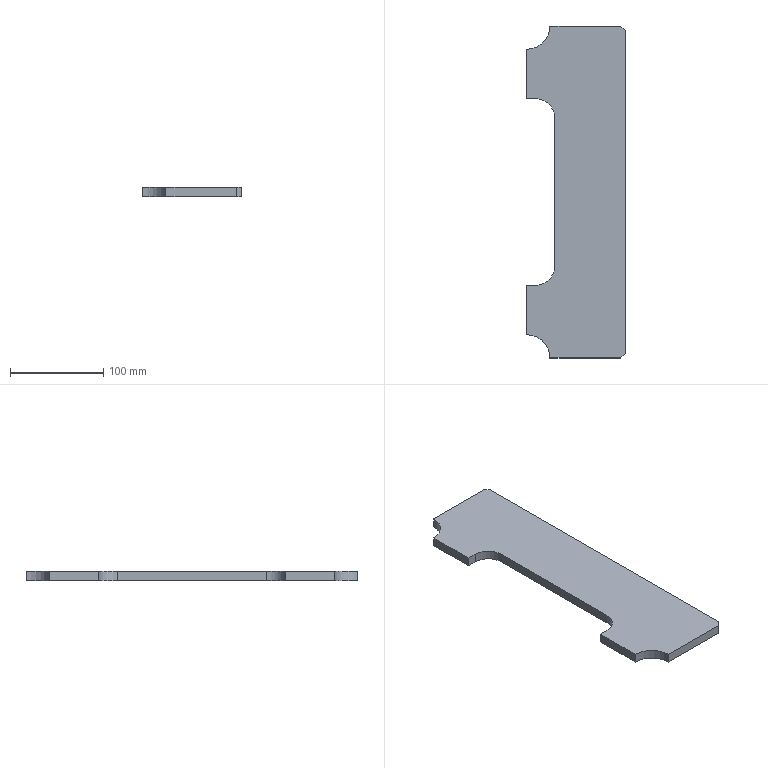Part | STEP file | VD-SYL0380DJ1006_1_1-9_VD-SYL03 | 1 solid | 16 faces | box 106 x 356 x 10 mm | volume 309009 mm3 | plane 12 | cylinder 4 | commonest cylinder face diameters 40 x2 50 x2
STEP:
#1=CARTESIAN_POINT('',(-53.,-153.,10.));
#2=VERTEX_POINT('',#1);
#3=CARTESIAN_POINT('',(-53.,-153.,0.));
#4=VERTEX_POINT('',#3);
#5=CARTESIAN_POINT('',(-53.,-153.,10.));
#6=DIRECTION('',(0.,0.,-1.));
#7=VECTOR('',#6,1000.);
#8=LINE('',#5,#7);
#9=EDGE_CURVE('',#2,#4,#8,.T.);
#10=ORIENTED_EDGE('',*,*,#9,.T.);
#11=CARTESIAN_POINT('',(-28.,-178.,0.));
#12=VERTEX_POINT('',#11);
#13=CARTESIAN_POINT('',(-53.,-178.,0.));
#14=DIRECTION('',(0.,0.,1.));
#15=DIRECTION('',(1.,0.,0.));
#16=AXIS2_PLACEMENT_3D('',#13,#14,#15);
#17=CIRCLE('',#16,25.);
#18=EDGE_CURVE('',#12,#4,#17,.T.);
#19=ORIENTED_EDGE('',*,*,#18,.F.);
#20=CARTESIAN_POINT('',(-28.,-178.,10.));
#21=VERTEX_POINT('',#20);
#22=CARTESIAN_POINT('',(-28.,-178.,0.));
#23=DIRECTION('',(0.,0.,1.));
#24=VECTOR('',#23,1000.);
#25=LINE('',#22,#24);
#26=EDGE_CURVE('',#12,#21,#25,.T.);
#27=ORIENTED_EDGE('',*,*,#26,.T.);
#28=CARTESIAN_POINT('',(-53.,-178.,10.));
#29=DIRECTION('',(0.,0.,-1.));
#30=DIRECTION('',(0.,1.,0.));
#31=AXIS2_PLACEMENT_3D('',#28,#29,#30);
#32=CIRCLE('',#31,25.);
#33=EDGE_CURVE('',#2,#21,#32,.T.);
#34=ORIENTED_EDGE('',*,*,#33,.F.);
#35=EDGE_LOOP('',(#10,#19,#27,#34));
#36=FACE_OUTER_BOUND('',#35,.T.);
#37=CARTESIAN_POINT('',(-53.,-178.,5.));
#38=DIRECTION('',(0.,0.,-1.));
#39=DIRECTION('',(-1.,0.,0.));
#40=AXIS2_PLACEMENT_3D('',#37,#38,#39);
#41=CYLINDRICAL_SURFACE('',#40,25.);
#42=ADVANCED_FACE('',(#36),#41,.F.);
#43=CARTESIAN_POINT('',(-43.,-100.,0.));
#44=VERTEX_POINT('',#43);
#45=CARTESIAN_POINT('',(-23.,-80.,0.));
#46=VERTEX_POINT('',#45);
#47=CARTESIAN_POINT('',(-43.,-80.,0.));
#48=DIRECTION('',(0.,0.,1.));
#49=DIRECTION('',(0.,-1.,0.));
#50=AXIS2_PLACEMENT_3D('',#47,#48,#49);
#51=CIRCLE('',#50,20.);
#52=EDGE_CURVE('',#44,#46,#51,.T.);
#53=ORIENTED_EDGE('',*,*,#52,.F.);
#54=CARTESIAN_POINT('',(-43.,-100.,10.));
#55=VERTEX_POINT('',#54);
#56=CARTESIAN_POINT('',(-43.,-100.,0.));
#57=DIRECTION('',(0.,0.,1.));
#58=VECTOR('',#57,1000.);
#59=LINE('',#56,#58);
#60=EDGE_CURVE('',#44,#55,#59,.T.);
#61=ORIENTED_EDGE('',*,*,#60,.T.);
#62=CARTESIAN_POINT('',(-23.,-80.,10.));
#63=VERTEX_POINT('',#62);
#64=CARTESIAN_POINT('',(-43.,-80.,10.));
#65=DIRECTION('',(0.,0.,-1.));
#66=DIRECTION('',(1.,0.,0.));
#67=AXIS2_PLACEMENT_3D('',#64,#65,#66);
#68=CIRCLE('',#67,20.);
#69=EDGE_CURVE('',#63,#55,#68,.T.);
#70=ORIENTED_EDGE('',*,*,#69,.F.);
#71=CARTESIAN_POINT('',(-23.,-80.,10.));
#72=DIRECTION('',(0.,0.,-1.));
#73=VECTOR('',#72,1000.);
#74=LINE('',#71,#73);
#75=EDGE_CURVE('',#63,#46,#74,.T.);
#76=ORIENTED_EDGE('',*,*,#75,.T.);
#77=EDGE_LOOP('',(#53,#61,#70,#76));
#78=FACE_OUTER_BOUND('',#77,.T.);
#79=CARTESIAN_POINT('',(-43.,-80.,-25.06));
#80=DIRECTION('',(0.,0.,1.));
#81=DIRECTION('',(1.,0.,0.));
#82=AXIS2_PLACEMENT_3D('',#79,#80,#81);
#83=CYLINDRICAL_SURFACE('',#82,20.);
#84=ADVANCED_FACE('',(#78),#83,.F.);
#85=CARTESIAN_POINT('',(-23.,80.,0.));
#86=VERTEX_POINT('',#85);
#87=CARTESIAN_POINT('',(-23.,80.,0.));
#88=DIRECTION('',(0.,-1.,0.));
#89=VECTOR('',#88,1000.);
#90=LINE('',#87,#89);
#91=EDGE_CURVE('',#86,#46,#90,.T.);
#92=ORIENTED_EDGE('',*,*,#91,.T.);
#93=ORIENTED_EDGE('',*,*,#75,.F.);
#94=CARTESIAN_POINT('',(-23.,80.,10.));
#95=VERTEX_POINT('',#94);
#96=CARTESIAN_POINT('',(-23.,-80.,10.));
#97=DIRECTION('',(0.,1.,0.));
#98=VECTOR('',#97,1000.);
#99=LINE('',#96,#98);
#100=EDGE_CURVE('',#63,#95,#99,.T.);
#101=ORIENTED_EDGE('',*,*,#100,.T.);
#102=CARTESIAN_POINT('',(-23.,80.,0.));
#103=DIRECTION('',(0.,0.,1.));
#104=VECTOR('',#103,1000.);
#105=LINE('',#102,#104);
#106=EDGE_CURVE('',#86,#95,#105,.T.);
#107=ORIENTED_EDGE('',*,*,#106,.F.);
#108=EDGE_LOOP('',(#92,#93,#101,#107));
#109=FACE_OUTER_BOUND('',#108,.T.);
#110=CARTESIAN_POINT('',(-23.,0.,5.));
#111=DIRECTION('',(1.,0.,0.));
#112=DIRECTION('',(0.,1.,0.));
#113=AXIS2_PLACEMENT_3D('',#110,#111,#112);
#114=PLANE('',#113);
#115=ADVANCED_FACE('',(#109),#114,.F.);
#116=CARTESIAN_POINT('',(-43.,100.,0.));
#117=VERTEX_POINT('',#116);
#118=CARTESIAN_POINT('',(-43.,80.,0.));
#119=DIRECTION('',(0.,0.,1.));
#120=DIRECTION('',(1.,0.,0.));
#121=AXIS2_PLACEMENT_3D('',#118,#119,#120);
#122=CIRCLE('',#121,20.);
#123=EDGE_CURVE('',#86,#117,#122,.T.);
#124=ORIENTED_EDGE('',*,*,#123,.F.);
#125=ORIENTED_EDGE('',*,*,#106,.T.);
#126=CARTESIAN_POINT('',(-43.,100.,10.));
#127=VERTEX_POINT('',#126);
#128=CARTESIAN_POINT('',(-43.,80.,10.));
#129=DIRECTION('',(0.,0.,-1.));
#130=DIRECTION('',(0.,1.,0.));
#131=AXIS2_PLACEMENT_3D('',#128,#129,#130);
#132=CIRCLE('',#131,20.);
#133=EDGE_CURVE('',#127,#95,#132,.T.);
#134=ORIENTED_EDGE('',*,*,#133,.F.);
#135=CARTESIAN_POINT('',(-43.,100.,10.));
#136=DIRECTION('',(0.,0.,-1.));
#137=VECTOR('',#136,1000.);
#138=LINE('',#135,#137);
#139=EDGE_CURVE('',#127,#117,#138,.T.);
#140=ORIENTED_EDGE('',*,*,#139,.T.);
#141=EDGE_LOOP('',(#124,#125,#134,#140));
#142=FACE_OUTER_BOUND('',#141,.T.);
#143=CARTESIAN_POINT('',(-43.,80.,-25.06));
#144=DIRECTION('',(0.,0.,1.));
#145=DIRECTION('',(1.,0.,0.));
#146=AXIS2_PLACEMENT_3D('',#143,#144,#145);
#147=CYLINDRICAL_SURFACE('',#146,20.);
#148=ADVANCED_FACE('',(#142),#147,.F.);
#149=CARTESIAN_POINT('',(-53.,100.,0.));
#150=VERTEX_POINT('',#149);
#151=CARTESIAN_POINT('',(-53.,100.,0.));
#152=DIRECTION('',(1.,0.,0.));
#153=VECTOR('',#152,1000.);
#154=LINE('',#151,#153);
#155=EDGE_CURVE('',#150,#117,#154,.T.);
#156=ORIENTED_EDGE('',*,*,#155,.T.);
#157=ORIENTED_EDGE('',*,*,#139,.F.);
#158=CARTESIAN_POINT('',(-53.,100.,10.));
#159=VERTEX_POINT('',#158);
#160=CARTESIAN_POINT('',(-43.,100.,10.));
#161=DIRECTION('',(-1.,0.,0.));
#162=VECTOR('',#161,1000.);
#163=LINE('',#160,#162);
#164=EDGE_CURVE('',#127,#159,#163,.T.);
#165=ORIENTED_EDGE('',*,*,#164,.T.);
#166=CARTESIAN_POINT('',(-53.,100.,10.));
#167=DIRECTION('',(0.,0.,-1.));
#168=VECTOR('',#167,1000.);
#169=LINE('',#166,#168);
#170=EDGE_CURVE('',#159,#150,#169,.T.);
#171=ORIENTED_EDGE('',*,*,#170,.T.);
#172=EDGE_LOOP('',(#156,#157,#165,#171));
#173=FACE_OUTER_BOUND('',#172,.T.);
#174=CARTESIAN_POINT('',(-38.,100.,5.));
#175=DIRECTION('',(0.,1.,0.));
#176=DIRECTION('',(1.,0.,0.));
#177=AXIS2_PLACEMENT_3D('',#174,#175,#176);
#178=PLANE('',#177);
#179=ADVANCED_FACE('',(#173),#178,.F.);
#180=CARTESIAN_POINT('',(-53.,153.,10.));
#181=VERTEX_POINT('',#180);
#182=CARTESIAN_POINT('',(-53.,100.,10.));
#183=DIRECTION('',(0.,1.,0.));
#184=VECTOR('',#183,1000.);
#185=LINE('',#182,#184);
#186=EDGE_CURVE('',#159,#181,#185,.T.);
#187=ORIENTED_EDGE('',*,*,#186,.T.);
#188=CARTESIAN_POINT('',(-53.,153.,0.));
#189=VERTEX_POINT('',#188);
#190=CARTESIAN_POINT('',(-53.,153.,0.));
#191=DIRECTION('',(0.,0.,1.));
#192=VECTOR('',#191,1000.);
#193=LINE('',#190,#192);
#194=EDGE_CURVE('',#189,#181,#193,.T.);
#195=ORIENTED_EDGE('',*,*,#194,.F.);
#196=CARTESIAN_POINT('',(-53.,153.,0.));
#197=DIRECTION('',(0.,-1.,0.));
#198=VECTOR('',#197,1000.);
#199=LINE('',#196,#198);
#200=EDGE_CURVE('',#189,#150,#199,.T.);
#201=ORIENTED_EDGE('',*,*,#200,.T.);
#202=ORIENTED_EDGE('',*,*,#170,.F.);
#203=EDGE_LOOP('',(#187,#195,#201,#202));
#204=FACE_OUTER_BOUND('',#203,.T.);
#205=CARTESIAN_POINT('',(-53.,0.,5.));
#206=DIRECTION('',(1.,0.,0.));
#207=DIRECTION('',(0.,1.,0.));
#208=AXIS2_PLACEMENT_3D('',#205,#206,#207);
#209=PLANE('',#208);
#210=ADVANCED_FACE('',(#204),#209,.F.);
#211=CARTESIAN_POINT('',(-28.,178.,10.));
#212=VERTEX_POINT('',#211);
#213=CARTESIAN_POINT('',(-28.,178.,0.));
#214=VERTEX_POINT('',#213);
#215=CARTESIAN_POINT('',(-28.,178.,10.));
#216=DIRECTION('',(0.,0.,-1.));
#217=VECTOR('',#216,1000.);
#218=LINE('',#215,#217);
#219=EDGE_CURVE('',#212,#214,#218,.T.);
#220=ORIENTED_EDGE('',*,*,#219,.T.);
#221=CARTESIAN_POINT('',(-53.,178.,0.));
#222=DIRECTION('',(0.,0.,1.));
#223=DIRECTION('',(0.,-1.,0.));
#224=AXIS2_PLACEMENT_3D('',#221,#222,#223);
#225=CIRCLE('',#224,25.);
#226=EDGE_CURVE('',#189,#214,#225,.T.);
#227=ORIENTED_EDGE('',*,*,#226,.F.);
#228=ORIENTED_EDGE('',*,*,#194,.T.);
#229=CARTESIAN_POINT('',(-53.,178.,10.));
#230=DIRECTION('',(0.,0.,-1.));
#231=DIRECTION('',(1.,0.,0.));
#232=AXIS2_PLACEMENT_3D('',#229,#230,#231);
#233=CIRCLE('',#232,25.);
#234=EDGE_CURVE('',#212,#181,#233,.T.);
#235=ORIENTED_EDGE('',*,*,#234,.F.);
#236=EDGE_LOOP('',(#220,#227,#228,#235));
#237=FACE_OUTER_BOUND('',#236,.T.);
#238=CARTESIAN_POINT('',(-53.,178.,5.));
#239=DIRECTION('',(0.,0.,-1.));
#240=DIRECTION('',(-1.,0.,0.));
#241=AXIS2_PLACEMENT_3D('',#238,#239,#240);
#242=CYLINDRICAL_SURFACE('',#241,25.);
#243=ADVANCED_FACE('',(#237),#242,.F.);
#244=CARTESIAN_POINT('',(53.,-173.,0.));
#245=VERTEX_POINT('',#244);
#246=CARTESIAN_POINT('',(53.,173.,0.));
#247=VERTEX_POINT('',#246);
#248=CARTESIAN_POINT('',(53.,-173.,0.));
#249=DIRECTION('',(0.,1.,0.));
#250=VECTOR('',#249,1000.);
#251=LINE('',#248,#250);
#252=EDGE_CURVE('',#245,#247,#251,.T.);
#253=ORIENTED_EDGE('',*,*,#252,.F.);
#254=CARTESIAN_POINT('',(48.,-178.,0.));
#255=VERTEX_POINT('',#254);
#256=CARTESIAN_POINT('',(53.,-173.,0.));
#257=DIRECTION('',(-0.7071,-0.7071,0.));
#258=VECTOR('',#257,1000.);
#259=LINE('',#256,#258);
#260=EDGE_CURVE('',#245,#255,#259,.T.);
#261=ORIENTED_EDGE('',*,*,#260,.T.);
#262=CARTESIAN_POINT('',(-28.,-178.,0.));
#263=DIRECTION('',(1.,0.,0.));
#264=VECTOR('',#263,1000.);
#265=LINE('',#262,#264);
#266=EDGE_CURVE('',#12,#255,#265,.T.);
#267=ORIENTED_EDGE('',*,*,#266,.F.);
#268=ORIENTED_EDGE('',*,*,#18,.T.);
#269=CARTESIAN_POINT('',(-53.,-100.,0.));
#270=VERTEX_POINT('',#269);
#271=CARTESIAN_POINT('',(-53.,-100.,0.));
#272=DIRECTION('',(0.,-1.,0.));
#273=VECTOR('',#272,1000.);
#274=LINE('',#271,#273);
#275=EDGE_CURVE('',#270,#4,#274,.T.);
#276=ORIENTED_EDGE('',*,*,#275,.F.);
#277=CARTESIAN_POINT('',(-53.,-100.,0.));
#278=DIRECTION('',(1.,0.,0.));
#279=VECTOR('',#278,1000.);
#280=LINE('',#277,#279);
#281=EDGE_CURVE('',#270,#44,#280,.T.);
#282=ORIENTED_EDGE('',*,*,#281,.T.);
#283=ORIENTED_EDGE('',*,*,#52,.T.);
#284=ORIENTED_EDGE('',*,*,#91,.F.);
#285=ORIENTED_EDGE('',*,*,#123,.T.);
#286=ORIENTED_EDGE('',*,*,#155,.F.);
#287=ORIENTED_EDGE('',*,*,#200,.F.);
#288=ORIENTED_EDGE('',*,*,#226,.T.);
#289=CARTESIAN_POINT('',(48.,178.,0.));
#290=VERTEX_POINT('',#289);
#291=CARTESIAN_POINT('',(48.,178.,0.));
#292=DIRECTION('',(-1.,0.,0.));
#293=VECTOR('',#292,1000.);
#294=LINE('',#291,#293);
#295=EDGE_CURVE('',#290,#214,#294,.T.);
#296=ORIENTED_EDGE('',*,*,#295,.F.);
#297=CARTESIAN_POINT('',(48.,178.,0.));
#298=DIRECTION('',(0.7071,-0.7071,0.));
#299=VECTOR('',#298,1000.);
#300=LINE('',#297,#299);
#301=EDGE_CURVE('',#290,#247,#300,.T.);
#302=ORIENTED_EDGE('',*,*,#301,.T.);
#303=EDGE_LOOP('',(#253,#261,#267,#268,#276,#282,#283,#284,#285,#286,#287,#288,#296,#302));
#304=FACE_OUTER_BOUND('',#303,.T.);
#305=CARTESIAN_POINT('',(0.,0.,0.));
#306=DIRECTION('',(0.,0.,1.));
#307=DIRECTION('',(1.,0.,0.));
#308=AXIS2_PLACEMENT_3D('',#305,#306,#307);
#309=PLANE('',#308);
#310=ADVANCED_FACE('',(#304),#309,.F.);
#311=CARTESIAN_POINT('',(48.,-178.,10.));
#312=VERTEX_POINT('',#311);
#313=CARTESIAN_POINT('',(48.,-178.,10.));
#314=DIRECTION('',(-1.,0.,0.));
#315=VECTOR('',#314,1000.);
#316=LINE('',#313,#315);
#317=EDGE_CURVE('',#312,#21,#316,.T.);
#318=ORIENTED_EDGE('',*,*,#317,.T.);
#319=ORIENTED_EDGE('',*,*,#26,.F.);
#320=ORIENTED_EDGE('',*,*,#266,.T.);
#321=CARTESIAN_POINT('',(48.,-178.,0.));
#322=DIRECTION('',(0.,0.,1.));
#323=VECTOR('',#322,1000.);
#324=LINE('',#321,#323);
#325=EDGE_CURVE('',#255,#312,#324,.T.);
#326=ORIENTED_EDGE('',*,*,#325,.T.);
#327=EDGE_LOOP('',(#318,#319,#320,#326));
#328=FACE_OUTER_BOUND('',#327,.T.);
#329=CARTESIAN_POINT('',(0.,-178.,5.));
#330=DIRECTION('',(0.,1.,0.));
#331=DIRECTION('',(1.,0.,0.));
#332=AXIS2_PLACEMENT_3D('',#329,#330,#331);
#333=PLANE('',#332);
#334=ADVANCED_FACE('',(#328),#333,.F.);
#335=ORIENTED_EDGE('',*,*,#260,.F.);
#336=CARTESIAN_POINT('',(53.,-173.,10.));
#337=VERTEX_POINT('',#336);
#338=CARTESIAN_POINT('',(53.,-173.,10.));
#339=DIRECTION('',(0.,0.,-1.));
#340=VECTOR('',#339,1000.);
#341=LINE('',#338,#340);
#342=EDGE_CURVE('',#337,#245,#341,.T.);
#343=ORIENTED_EDGE('',*,*,#342,.F.);
#344=CARTESIAN_POINT('',(48.,-178.,10.));
#345=DIRECTION('',(0.7071,0.7071,0.));
#346=VECTOR('',#345,1000.);
#347=LINE('',#344,#346);
#348=EDGE_CURVE('',#312,#337,#347,.T.);
#349=ORIENTED_EDGE('',*,*,#348,.F.);
#350=ORIENTED_EDGE('',*,*,#325,.F.);
#351=EDGE_LOOP('',(#335,#343,#349,#350));
#352=FACE_OUTER_BOUND('',#351,.T.);
#353=CARTESIAN_POINT('',(50.5,-175.5,5.));
#354=DIRECTION('',(0.7071,-0.7071,0.));
#355=DIRECTION('',(0.,0.,-1.));
#356=AXIS2_PLACEMENT_3D('',#353,#354,#355);
#357=PLANE('',#356);
#358=ADVANCED_FACE('',(#352),#357,.T.);
#359=ORIENTED_EDGE('',*,*,#252,.T.);
#360=CARTESIAN_POINT('',(53.,173.,10.));
#361=VERTEX_POINT('',#360);
#362=CARTESIAN_POINT('',(53.,173.,0.));
#363=DIRECTION('',(0.,0.,1.));
#364=VECTOR('',#363,1000.);
#365=LINE('',#362,#364);
#366=EDGE_CURVE('',#247,#361,#365,.T.);
#367=ORIENTED_EDGE('',*,*,#366,.T.);
#368=CARTESIAN_POINT('',(53.,173.,10.));
#369=DIRECTION('',(0.,-1.,0.));
#370=VECTOR('',#369,1000.);
#371=LINE('',#368,#370);
#372=EDGE_CURVE('',#361,#337,#371,.T.);
#373=ORIENTED_EDGE('',*,*,#372,.T.);
#374=ORIENTED_EDGE('',*,*,#342,.T.);
#375=EDGE_LOOP('',(#359,#367,#373,#374));
#376=FACE_OUTER_BOUND('',#375,.T.);
#377=CARTESIAN_POINT('',(53.,0.,5.));
#378=DIRECTION('',(-1.,0.,0.));
#379=DIRECTION('',(0.,0.,1.));
#380=AXIS2_PLACEMENT_3D('',#377,#378,#379);
#381=PLANE('',#380);
#382=ADVANCED_FACE('',(#376),#381,.F.);
#383=ORIENTED_EDGE('',*,*,#301,.F.);
#384=CARTESIAN_POINT('',(48.,178.,10.));
#385=VERTEX_POINT('',#384);
#386=CARTESIAN_POINT('',(48.,178.,10.));
#387=DIRECTION('',(0.,0.,-1.));
#388=VECTOR('',#387,1000.);
#389=LINE('',#386,#388);
#390=EDGE_CURVE('',#385,#290,#389,.T.);
#391=ORIENTED_EDGE('',*,*,#390,.F.);
#392=CARTESIAN_POINT('',(53.,173.,10.));
#393=DIRECTION('',(-0.7071,0.7071,0.));
#394=VECTOR('',#393,1000.);
#395=LINE('',#392,#394);
#396=EDGE_CURVE('',#361,#385,#395,.T.);
#397=ORIENTED_EDGE('',*,*,#396,.F.);
#398=ORIENTED_EDGE('',*,*,#366,.F.);
#399=EDGE_LOOP('',(#383,#391,#397,#398));
#400=FACE_OUTER_BOUND('',#399,.T.);
#401=CARTESIAN_POINT('',(50.5,175.5,5.));
#402=DIRECTION('',(0.7071,0.7071,0.));
#403=DIRECTION('',(0.,0.,-1.));
#404=AXIS2_PLACEMENT_3D('',#401,#402,#403);
#405=PLANE('',#404);
#406=ADVANCED_FACE('',(#400),#405,.T.);
#407=ORIENTED_EDGE('',*,*,#295,.T.);
#408=ORIENTED_EDGE('',*,*,#219,.F.);
#409=CARTESIAN_POINT('',(-28.,178.,10.));
#410=DIRECTION('',(1.,0.,0.));
#411=VECTOR('',#410,1000.);
#412=LINE('',#409,#411);
#413=EDGE_CURVE('',#212,#385,#412,.T.);
#414=ORIENTED_EDGE('',*,*,#413,.T.);
#415=ORIENTED_EDGE('',*,*,#390,.T.);
#416=EDGE_LOOP('',(#407,#408,#414,#415));
#417=FACE_OUTER_BOUND('',#416,.T.);
#418=CARTESIAN_POINT('',(0.,178.,5.));
#419=DIRECTION('',(0.,-1.,0.));
#420=DIRECTION('',(0.,0.,-1.));
#421=AXIS2_PLACEMENT_3D('',#418,#419,#420);
#422=PLANE('',#421);
#423=ADVANCED_FACE('',(#417),#422,.F.);
#424=ORIENTED_EDGE('',*,*,#234,.T.);
#425=ORIENTED_EDGE('',*,*,#186,.F.);
#426=ORIENTED_EDGE('',*,*,#164,.F.);
#427=ORIENTED_EDGE('',*,*,#133,.T.);
#428=ORIENTED_EDGE('',*,*,#100,.F.);
#429=ORIENTED_EDGE('',*,*,#69,.T.);
#430=CARTESIAN_POINT('',(-53.,-100.,10.));
#431=VERTEX_POINT('',#430);
#432=CARTESIAN_POINT('',(-53.,-100.,10.));
#433=DIRECTION('',(1.,0.,0.));
#434=VECTOR('',#433,1000.);
#435=LINE('',#432,#434);
#436=EDGE_CURVE('',#431,#55,#435,.T.);
#437=ORIENTED_EDGE('',*,*,#436,.F.);
#438=CARTESIAN_POINT('',(-53.,-153.,10.));
#439=DIRECTION('',(0.,1.,0.));
#440=VECTOR('',#439,1000.);
#441=LINE('',#438,#440);
#442=EDGE_CURVE('',#2,#431,#441,.T.);
#443=ORIENTED_EDGE('',*,*,#442,.F.);
#444=ORIENTED_EDGE('',*,*,#33,.T.);
#445=ORIENTED_EDGE('',*,*,#317,.F.);
#446=ORIENTED_EDGE('',*,*,#348,.T.);
#447=ORIENTED_EDGE('',*,*,#372,.F.);
#448=ORIENTED_EDGE('',*,*,#396,.T.);
#449=ORIENTED_EDGE('',*,*,#413,.F.);
#450=EDGE_LOOP('',(#424,#425,#426,#427,#428,#429,#437,#443,#444,#445,#446,#447,#448,#449));
#451=FACE_OUTER_BOUND('',#450,.T.);
#452=CARTESIAN_POINT('',(0.,0.,10.));
#453=DIRECTION('',(0.,0.,1.));
#454=DIRECTION('',(1.,0.,0.));
#455=AXIS2_PLACEMENT_3D('',#452,#453,#454);
#456=PLANE('',#455);
#457=ADVANCED_FACE('',(#451),#456,.T.);
#458=ORIENTED_EDGE('',*,*,#60,.F.);
#459=ORIENTED_EDGE('',*,*,#281,.F.);
#460=CARTESIAN_POINT('',(-53.,-100.,10.));
#461=DIRECTION('',(0.,0.,-1.));
#462=VECTOR('',#461,1000.);
#463=LINE('',#460,#462);
#464=EDGE_CURVE('',#431,#270,#463,.T.);
#465=ORIENTED_EDGE('',*,*,#464,.F.);
#466=ORIENTED_EDGE('',*,*,#436,.T.);
#467=EDGE_LOOP('',(#458,#459,#465,#466));
#468=FACE_OUTER_BOUND('',#467,.T.);
#469=CARTESIAN_POINT('',(-38.,-100.,5.));
#470=DIRECTION('',(0.,1.,0.));
#471=DIRECTION('',(1.,0.,0.));
#472=AXIS2_PLACEMENT_3D('',#469,#470,#471);
#473=PLANE('',#472);
#474=ADVANCED_FACE('',(#468),#473,.T.);
#475=ORIENTED_EDGE('',*,*,#275,.T.);
#476=ORIENTED_EDGE('',*,*,#9,.F.);
#477=ORIENTED_EDGE('',*,*,#442,.T.);
#478=ORIENTED_EDGE('',*,*,#464,.T.);
#479=EDGE_LOOP('',(#475,#476,#477,#478));
#480=FACE_OUTER_BOUND('',#479,.T.);
#481=CARTESIAN_POINT('',(-53.,0.,5.));
#482=DIRECTION('',(1.,0.,0.));
#483=DIRECTION('',(0.,1.,0.));
#484=AXIS2_PLACEMENT_3D('',#481,#482,#483);
#485=PLANE('',#484);
#486=ADVANCED_FACE('',(#480),#485,.F.);
#487=CLOSED_SHELL('',(#42,#84,#115,#148,#179,#210,#243,#310,#334,#358,#382,#406,#423,#457,#474,#486));
#488=MANIFOLD_SOLID_BREP('',#487);
#489=CARTESIAN_POINT('',(0.,0.,0.));
#490=DIRECTION('',(0.,0.,1.));
#491=DIRECTION('',(1.,0.,0.));
#492=AXIS2_PLACEMENT_3D('',#489,#490,#491);
#493=(LENGTH_UNIT()NAMED_UNIT(*)SI_UNIT(.MILLI.,.METRE.));
#494=UNCERTAINTY_MEASURE_WITH_UNIT(LENGTH_MEASURE(0.00001),#493,'','');
#495=(NAMED_UNIT(*)PLANE_ANGLE_UNIT()SI_UNIT($,.RADIAN.));
#496=(NAMED_UNIT(*)SI_UNIT($,.STERADIAN.)SOLID_ANGLE_UNIT());
#497=(GEOMETRIC_REPRESENTATION_CONTEXT(3)GLOBAL_UNCERTAINTY_ASSIGNED_CONTEXT((#494))GLOBAL_UNIT_ASSIGNED_CONTEXT((#493,#495,#496))REPRESENTATION_CONTEXT('',''));
#498=ADVANCED_BREP_SHAPE_REPRESENTATION('',(#488,#492),#497);